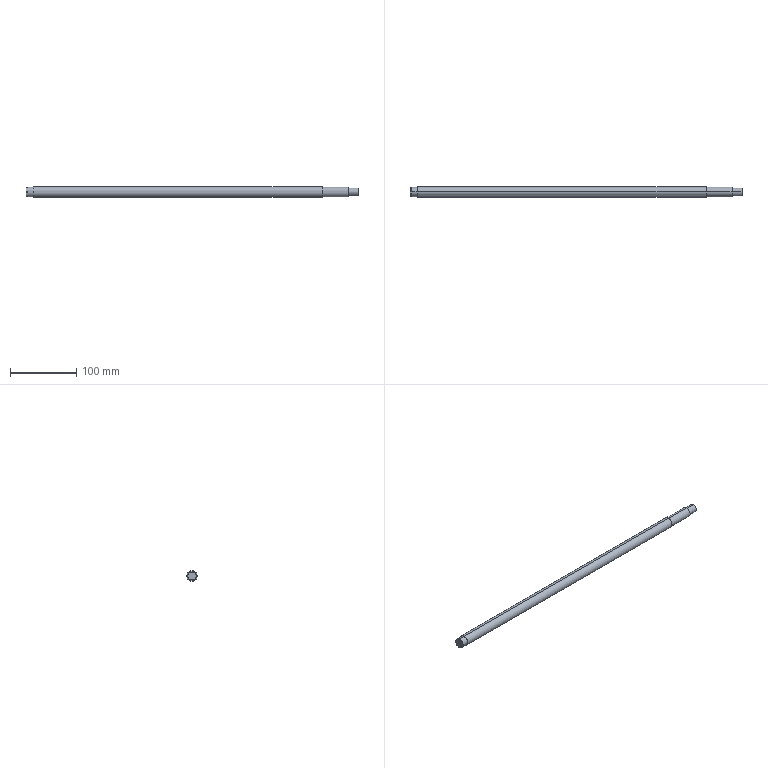Part | SolidWorks | features BaseBody 1 | 1 solid | 19 faces | box 500 x 16 x 16 mm | volume 97769 mm3 | cylinder 12 | plane 7 | commonest cylinder face diameters 14.3 x4 12 x2 12.3 x2 15 x2 16 x2
STEP:
#1=CARTESIAN_POINT('',(446.,0.,8.));
#2=VERTEX_POINT('',#1);
#3=CARTESIAN_POINT('',(446.,0.,-8.));
#4=VERTEX_POINT('',#3);
#5=CARTESIAN_POINT('',(446.,0.,0.));
#6=DIRECTION('',(-1.,0.,0.));
#7=DIRECTION('',(0.,0.,1.));
#8=AXIS2_PLACEMENT_3D('',#5,#6,#7);
#9=CIRCLE('',#8,8.);
#10=EDGE_CURVE('',#2,#4,#9,.T.);
#11=ORIENTED_EDGE('',*,*,#10,.T.);
#12=CARTESIAN_POINT('',(11.,0.,-8.));
#13=VERTEX_POINT('',#12);
#14=CARTESIAN_POINT('',(-271.923,0.,-8.));
#15=DIRECTION('',(-1.,0.,0.));
#16=VECTOR('',#15,1000.);
#17=LINE('',#14,#16);
#18=EDGE_CURVE('',#4,#13,#17,.T.);
#19=ORIENTED_EDGE('',*,*,#18,.T.);
#20=CARTESIAN_POINT('',(11.,0.,8.));
#21=VERTEX_POINT('',#20);
#22=CARTESIAN_POINT('',(11.,0.,0.));
#23=DIRECTION('',(1.,0.,0.));
#24=DIRECTION('',(0.,0.,1.));
#25=AXIS2_PLACEMENT_3D('',#22,#23,#24);
#26=CIRCLE('',#25,8.);
#27=EDGE_CURVE('',#13,#21,#26,.T.);
#28=ORIENTED_EDGE('',*,*,#27,.T.);
#29=CARTESIAN_POINT('',(-271.923,0.,8.));
#30=DIRECTION('',(-1.,0.,0.));
#31=VECTOR('',#30,1000.);
#32=LINE('',#29,#31);
#33=EDGE_CURVE('',#2,#21,#32,.T.);
#34=ORIENTED_EDGE('',*,*,#33,.F.);
#35=EDGE_LOOP('',(#11,#19,#28,#34));
#36=FACE_OUTER_BOUND('',#35,.T.);
#37=CARTESIAN_POINT('',(-271.923,0.,0.));
#38=DIRECTION('',(-1.,0.,0.));
#39=DIRECTION('',(0.,0.,1.));
#40=AXIS2_PLACEMENT_3D('',#37,#38,#39);
#41=CYLINDRICAL_SURFACE('',#40,8.);
#42=ADVANCED_FACE('',(#36),#41,.T.);
#43=CARTESIAN_POINT('',(11.,0.,7.15));
#44=VERTEX_POINT('',#43);
#45=CARTESIAN_POINT('',(11.,0.,-7.15));
#46=VERTEX_POINT('',#45);
#47=CARTESIAN_POINT('',(11.,0.,0.));
#48=DIRECTION('',(-1.,0.,0.));
#49=DIRECTION('',(0.,0.,1.));
#50=AXIS2_PLACEMENT_3D('',#47,#48,#49);
#51=CIRCLE('',#50,7.15);
#52=EDGE_CURVE('',#44,#46,#51,.T.);
#53=ORIENTED_EDGE('',*,*,#52,.T.);
#54=CARTESIAN_POINT('',(2.,0.,-7.15));
#55=VERTEX_POINT('',#54);
#56=CARTESIAN_POINT('',(-271.923,0.,-7.15));
#57=DIRECTION('',(-1.,0.,0.));
#58=VECTOR('',#57,1000.);
#59=LINE('',#56,#58);
#60=EDGE_CURVE('',#46,#55,#59,.T.);
#61=ORIENTED_EDGE('',*,*,#60,.T.);
#62=CARTESIAN_POINT('',(2.,0.,7.15));
#63=VERTEX_POINT('',#62);
#64=CARTESIAN_POINT('',(2.,0.,0.));
#65=DIRECTION('',(1.,0.,0.));
#66=DIRECTION('',(0.,0.,1.));
#67=AXIS2_PLACEMENT_3D('',#64,#65,#66);
#68=CIRCLE('',#67,7.15);
#69=EDGE_CURVE('',#55,#63,#68,.T.);
#70=ORIENTED_EDGE('',*,*,#69,.T.);
#71=CARTESIAN_POINT('',(-271.923,0.,7.15));
#72=DIRECTION('',(-1.,0.,0.));
#73=VECTOR('',#72,1000.);
#74=LINE('',#71,#73);
#75=EDGE_CURVE('',#44,#63,#74,.T.);
#76=ORIENTED_EDGE('',*,*,#75,.F.);
#77=EDGE_LOOP('',(#53,#61,#70,#76));
#78=FACE_OUTER_BOUND('',#77,.T.);
#79=CARTESIAN_POINT('',(-271.923,0.,0.));
#80=DIRECTION('',(-1.,0.,0.));
#81=DIRECTION('',(0.,0.,1.));
#82=AXIS2_PLACEMENT_3D('',#79,#80,#81);
#83=CYLINDRICAL_SURFACE('',#82,7.15);
#84=ADVANCED_FACE('',(#78),#83,.T.);
#85=CARTESIAN_POINT('',(485.,0.,7.5));
#86=VERTEX_POINT('',#85);
#87=CARTESIAN_POINT('',(485.,0.,-7.5));
#88=VERTEX_POINT('',#87);
#89=CARTESIAN_POINT('',(485.,0.,0.));
#90=DIRECTION('',(-1.,0.,0.));
#91=DIRECTION('',(0.,0.,1.));
#92=AXIS2_PLACEMENT_3D('',#89,#90,#91);
#93=CIRCLE('',#92,7.5);
#94=EDGE_CURVE('',#86,#88,#93,.T.);
#95=ORIENTED_EDGE('',*,*,#94,.T.);
#96=CARTESIAN_POINT('',(446.,0.,-7.5));
#97=VERTEX_POINT('',#96);
#98=CARTESIAN_POINT('',(-271.923,0.,-7.5));
#99=DIRECTION('',(-1.,0.,0.));
#100=VECTOR('',#99,1000.);
#101=LINE('',#98,#100);
#102=EDGE_CURVE('',#88,#97,#101,.T.);
#103=ORIENTED_EDGE('',*,*,#102,.T.);
#104=CARTESIAN_POINT('',(446.,0.,7.5));
#105=VERTEX_POINT('',#104);
#106=CARTESIAN_POINT('',(446.,0.,0.));
#107=DIRECTION('',(1.,0.,0.));
#108=DIRECTION('',(0.,0.,1.));
#109=AXIS2_PLACEMENT_3D('',#106,#107,#108);
#110=CIRCLE('',#109,7.5);
#111=EDGE_CURVE('',#97,#105,#110,.T.);
#112=ORIENTED_EDGE('',*,*,#111,.T.);
#113=CARTESIAN_POINT('',(-271.923,0.,7.5));
#114=DIRECTION('',(-1.,0.,0.));
#115=VECTOR('',#114,1000.);
#116=LINE('',#113,#115);
#117=EDGE_CURVE('',#86,#105,#116,.T.);
#118=ORIENTED_EDGE('',*,*,#117,.F.);
#119=EDGE_LOOP('',(#95,#103,#112,#118));
#120=FACE_OUTER_BOUND('',#119,.T.);
#121=CARTESIAN_POINT('',(-271.923,0.,0.));
#122=DIRECTION('',(-1.,0.,0.));
#123=DIRECTION('',(0.,0.,1.));
#124=AXIS2_PLACEMENT_3D('',#121,#122,#123);
#125=CYLINDRICAL_SURFACE('',#124,7.5);
#126=ADVANCED_FACE('',(#120),#125,.T.);
#127=CARTESIAN_POINT('',(2.,0.,6.15));
#128=VERTEX_POINT('',#127);
#129=CARTESIAN_POINT('',(2.,0.,-6.15));
#130=VERTEX_POINT('',#129);
#131=CARTESIAN_POINT('',(2.,0.,0.));
#132=DIRECTION('',(-1.,0.,0.));
#133=DIRECTION('',(0.,0.,1.));
#134=AXIS2_PLACEMENT_3D('',#131,#132,#133);
#135=CIRCLE('',#134,6.15);
#136=EDGE_CURVE('',#128,#130,#135,.T.);
#137=ORIENTED_EDGE('',*,*,#136,.T.);
#138=CARTESIAN_POINT('',(0.85,0.,-6.15));
#139=VERTEX_POINT('',#138);
#140=CARTESIAN_POINT('',(-271.923,0.,-6.15));
#141=DIRECTION('',(-1.,0.,0.));
#142=VECTOR('',#141,1000.);
#143=LINE('',#140,#142);
#144=EDGE_CURVE('',#130,#139,#143,.T.);
#145=ORIENTED_EDGE('',*,*,#144,.T.);
#146=CARTESIAN_POINT('',(0.85,0.,6.15));
#147=VERTEX_POINT('',#146);
#148=CARTESIAN_POINT('',(0.85,0.,0.));
#149=DIRECTION('',(1.,0.,0.));
#150=DIRECTION('',(0.,0.,1.));
#151=AXIS2_PLACEMENT_3D('',#148,#149,#150);
#152=CIRCLE('',#151,6.15);
#153=EDGE_CURVE('',#139,#147,#152,.T.);
#154=ORIENTED_EDGE('',*,*,#153,.T.);
#155=CARTESIAN_POINT('',(-271.923,0.,6.15));
#156=DIRECTION('',(-1.,0.,0.));
#157=VECTOR('',#156,1000.);
#158=LINE('',#155,#157);
#159=EDGE_CURVE('',#128,#147,#158,.T.);
#160=ORIENTED_EDGE('',*,*,#159,.F.);
#161=EDGE_LOOP('',(#137,#145,#154,#160));
#162=FACE_OUTER_BOUND('',#161,.T.);
#163=CARTESIAN_POINT('',(-271.923,0.,0.));
#164=DIRECTION('',(-1.,0.,0.));
#165=DIRECTION('',(0.,0.,1.));
#166=AXIS2_PLACEMENT_3D('',#163,#164,#165);
#167=CYLINDRICAL_SURFACE('',#166,6.15);
#168=ADVANCED_FACE('',(#162),#167,.T.);
#169=CARTESIAN_POINT('',(500.,0.,6.));
#170=VERTEX_POINT('',#169);
#171=CARTESIAN_POINT('',(500.,0.,-6.));
#172=VERTEX_POINT('',#171);
#173=CARTESIAN_POINT('',(500.,0.,0.));
#174=DIRECTION('',(-1.,0.,0.));
#175=DIRECTION('',(0.,0.,1.));
#176=AXIS2_PLACEMENT_3D('',#173,#174,#175);
#177=CIRCLE('',#176,6.);
#178=EDGE_CURVE('',#170,#172,#177,.T.);
#179=ORIENTED_EDGE('',*,*,#178,.T.);
#180=CARTESIAN_POINT('',(485.,0.,-6.));
#181=VERTEX_POINT('',#180);
#182=CARTESIAN_POINT('',(-271.923,0.,-6.));
#183=DIRECTION('',(-1.,0.,0.));
#184=VECTOR('',#183,1000.);
#185=LINE('',#182,#184);
#186=EDGE_CURVE('',#172,#181,#185,.T.);
#187=ORIENTED_EDGE('',*,*,#186,.T.);
#188=CARTESIAN_POINT('',(485.,0.,6.));
#189=VERTEX_POINT('',#188);
#190=CARTESIAN_POINT('',(485.,0.,0.));
#191=DIRECTION('',(1.,0.,0.));
#192=DIRECTION('',(0.,0.,1.));
#193=AXIS2_PLACEMENT_3D('',#190,#191,#192);
#194=CIRCLE('',#193,6.);
#195=EDGE_CURVE('',#181,#189,#194,.T.);
#196=ORIENTED_EDGE('',*,*,#195,.T.);
#197=CARTESIAN_POINT('',(-271.923,0.,6.));
#198=DIRECTION('',(-1.,0.,0.));
#199=VECTOR('',#198,1000.);
#200=LINE('',#197,#199);
#201=EDGE_CURVE('',#170,#189,#200,.T.);
#202=ORIENTED_EDGE('',*,*,#201,.F.);
#203=EDGE_LOOP('',(#179,#187,#196,#202));
#204=FACE_OUTER_BOUND('',#203,.T.);
#205=CARTESIAN_POINT('',(-271.923,0.,0.));
#206=DIRECTION('',(-1.,0.,0.));
#207=DIRECTION('',(0.,0.,1.));
#208=AXIS2_PLACEMENT_3D('',#205,#206,#207);
#209=CYLINDRICAL_SURFACE('',#208,6.);
#210=ADVANCED_FACE('',(#204),#209,.T.);
#211=CARTESIAN_POINT('',(0.85,0.,7.15));
#212=VERTEX_POINT('',#211);
#213=CARTESIAN_POINT('',(0.85,0.,-7.15));
#214=VERTEX_POINT('',#213);
#215=CARTESIAN_POINT('',(0.85,0.,0.));
#216=DIRECTION('',(-1.,0.,0.));
#217=DIRECTION('',(0.,0.,1.));
#218=AXIS2_PLACEMENT_3D('',#215,#216,#217);
#219=CIRCLE('',#218,7.15);
#220=EDGE_CURVE('',#212,#214,#219,.T.);
#221=ORIENTED_EDGE('',*,*,#220,.T.);
#222=CARTESIAN_POINT('',(0.,0.,-7.15));
#223=VERTEX_POINT('',#222);
#224=CARTESIAN_POINT('',(-271.923,0.,-7.15));
#225=DIRECTION('',(-1.,0.,0.));
#226=VECTOR('',#225,1000.);
#227=LINE('',#224,#226);
#228=EDGE_CURVE('',#214,#223,#227,.T.);
#229=ORIENTED_EDGE('',*,*,#228,.T.);
#230=CARTESIAN_POINT('',(0.,0.,7.15));
#231=VERTEX_POINT('',#230);
#232=CARTESIAN_POINT('',(0.,0.,0.));
#233=DIRECTION('',(1.,0.,0.));
#234=DIRECTION('',(0.,0.,1.));
#235=AXIS2_PLACEMENT_3D('',#232,#233,#234);
#236=CIRCLE('',#235,7.15);
#237=EDGE_CURVE('',#223,#231,#236,.T.);
#238=ORIENTED_EDGE('',*,*,#237,.T.);
#239=CARTESIAN_POINT('',(-271.923,0.,7.15));
#240=DIRECTION('',(-1.,0.,0.));
#241=VECTOR('',#240,1000.);
#242=LINE('',#239,#241);
#243=EDGE_CURVE('',#212,#231,#242,.T.);
#244=ORIENTED_EDGE('',*,*,#243,.F.);
#245=EDGE_LOOP('',(#221,#229,#238,#244));
#246=FACE_OUTER_BOUND('',#245,.T.);
#247=CARTESIAN_POINT('',(-271.923,0.,0.));
#248=DIRECTION('',(-1.,0.,0.));
#249=DIRECTION('',(0.,0.,1.));
#250=AXIS2_PLACEMENT_3D('',#247,#248,#249);
#251=CYLINDRICAL_SURFACE('',#250,7.15);
#252=ADVANCED_FACE('',(#246),#251,.T.);
#253=ORIENTED_EDGE('',*,*,#18,.F.);
#254=CARTESIAN_POINT('',(446.,0.,0.));
#255=DIRECTION('',(-1.,0.,0.));
#256=DIRECTION('',(0.,0.,1.));
#257=AXIS2_PLACEMENT_3D('',#254,#255,#256);
#258=CIRCLE('',#257,8.);
#259=EDGE_CURVE('',#4,#2,#258,.T.);
#260=ORIENTED_EDGE('',*,*,#259,.T.);
#261=ORIENTED_EDGE('',*,*,#33,.T.);
#262=CARTESIAN_POINT('',(11.,0.,0.));
#263=DIRECTION('',(1.,0.,0.));
#264=DIRECTION('',(0.,0.,1.));
#265=AXIS2_PLACEMENT_3D('',#262,#263,#264);
#266=CIRCLE('',#265,8.);
#267=EDGE_CURVE('',#21,#13,#266,.T.);
#268=ORIENTED_EDGE('',*,*,#267,.T.);
#269=EDGE_LOOP('',(#253,#260,#261,#268));
#270=FACE_OUTER_BOUND('',#269,.T.);
#271=CARTESIAN_POINT('',(-271.923,0.,0.));
#272=DIRECTION('',(-1.,0.,0.));
#273=DIRECTION('',(0.,0.,1.));
#274=AXIS2_PLACEMENT_3D('',#271,#272,#273);
#275=CYLINDRICAL_SURFACE('',#274,8.);
#276=ADVANCED_FACE('',(#270),#275,.T.);
#277=ORIENTED_EDGE('',*,*,#267,.F.);
#278=ORIENTED_EDGE('',*,*,#27,.F.);
#279=EDGE_LOOP('',(#277,#278));
#280=FACE_OUTER_BOUND('',#279,.T.);
#281=ORIENTED_EDGE('',*,*,#52,.F.);
#282=CARTESIAN_POINT('',(11.,0.,0.));
#283=DIRECTION('',(-1.,0.,0.));
#284=DIRECTION('',(0.,0.,1.));
#285=AXIS2_PLACEMENT_3D('',#282,#283,#284);
#286=CIRCLE('',#285,7.15);
#287=EDGE_CURVE('',#46,#44,#286,.T.);
#288=ORIENTED_EDGE('',*,*,#287,.F.);
#289=EDGE_LOOP('',(#281,#288));
#290=FACE_BOUND('',#289,.T.);
#291=CARTESIAN_POINT('',(11.,7.15,0.));
#292=DIRECTION('',(1.,0.,0.));
#293=DIRECTION('',(0.,0.,-1.));
#294=AXIS2_PLACEMENT_3D('',#291,#292,#293);
#295=PLANE('',#294);
#296=ADVANCED_FACE('',(#280,#290),#295,.F.);
#297=CARTESIAN_POINT('',(446.,0.,0.));
#298=DIRECTION('',(1.,0.,0.));
#299=DIRECTION('',(0.,0.,1.));
#300=AXIS2_PLACEMENT_3D('',#297,#298,#299);
#301=CIRCLE('',#300,7.5);
#302=EDGE_CURVE('',#105,#97,#301,.T.);
#303=ORIENTED_EDGE('',*,*,#302,.F.);
#304=ORIENTED_EDGE('',*,*,#111,.F.);
#305=EDGE_LOOP('',(#303,#304));
#306=FACE_BOUND('',#305,.T.);
#307=ORIENTED_EDGE('',*,*,#10,.F.);
#308=ORIENTED_EDGE('',*,*,#259,.F.);
#309=EDGE_LOOP('',(#307,#308));
#310=FACE_OUTER_BOUND('',#309,.T.);
#311=CARTESIAN_POINT('',(446.,8.,0.));
#312=DIRECTION('',(-1.,0.,0.));
#313=DIRECTION('',(0.,0.,1.));
#314=AXIS2_PLACEMENT_3D('',#311,#312,#313);
#315=PLANE('',#314);
#316=ADVANCED_FACE('',(#306,#310),#315,.F.);
#317=ORIENTED_EDGE('',*,*,#60,.F.);
#318=ORIENTED_EDGE('',*,*,#287,.T.);
#319=ORIENTED_EDGE('',*,*,#75,.T.);
#320=CARTESIAN_POINT('',(2.,0.,0.));
#321=DIRECTION('',(1.,0.,0.));
#322=DIRECTION('',(0.,0.,1.));
#323=AXIS2_PLACEMENT_3D('',#320,#321,#322);
#324=CIRCLE('',#323,7.15);
#325=EDGE_CURVE('',#63,#55,#324,.T.);
#326=ORIENTED_EDGE('',*,*,#325,.T.);
#327=EDGE_LOOP('',(#317,#318,#319,#326));
#328=FACE_OUTER_BOUND('',#327,.T.);
#329=CARTESIAN_POINT('',(-271.923,0.,0.));
#330=DIRECTION('',(-1.,0.,0.));
#331=DIRECTION('',(0.,0.,1.));
#332=AXIS2_PLACEMENT_3D('',#329,#330,#331);
#333=CYLINDRICAL_SURFACE('',#332,7.15);
#334=ADVANCED_FACE('',(#328),#333,.T.);
#335=ORIENTED_EDGE('',*,*,#102,.F.);
#336=CARTESIAN_POINT('',(485.,0.,0.));
#337=DIRECTION('',(-1.,0.,0.));
#338=DIRECTION('',(0.,0.,1.));
#339=AXIS2_PLACEMENT_3D('',#336,#337,#338);
#340=CIRCLE('',#339,7.5);
#341=EDGE_CURVE('',#88,#86,#340,.T.);
#342=ORIENTED_EDGE('',*,*,#341,.T.);
#343=ORIENTED_EDGE('',*,*,#117,.T.);
#344=ORIENTED_EDGE('',*,*,#302,.T.);
#345=EDGE_LOOP('',(#335,#342,#343,#344));
#346=FACE_OUTER_BOUND('',#345,.T.);
#347=CARTESIAN_POINT('',(-271.923,0.,0.));
#348=DIRECTION('',(-1.,0.,0.));
#349=DIRECTION('',(0.,0.,1.));
#350=AXIS2_PLACEMENT_3D('',#347,#348,#349);
#351=CYLINDRICAL_SURFACE('',#350,7.5);
#352=ADVANCED_FACE('',(#346),#351,.T.);
#353=ORIENTED_EDGE('',*,*,#325,.F.);
#354=ORIENTED_EDGE('',*,*,#69,.F.);
#355=EDGE_LOOP('',(#353,#354));
#356=FACE_OUTER_BOUND('',#355,.T.);
#357=ORIENTED_EDGE('',*,*,#136,.F.);
#358=CARTESIAN_POINT('',(2.,0.,0.));
#359=DIRECTION('',(-1.,0.,0.));
#360=DIRECTION('',(0.,0.,1.));
#361=AXIS2_PLACEMENT_3D('',#358,#359,#360);
#362=CIRCLE('',#361,6.15);
#363=EDGE_CURVE('',#130,#128,#362,.T.);
#364=ORIENTED_EDGE('',*,*,#363,.F.);
#365=EDGE_LOOP('',(#357,#364));
#366=FACE_BOUND('',#365,.T.);
#367=CARTESIAN_POINT('',(2.,6.15,0.));
#368=DIRECTION('',(1.,0.,0.));
#369=DIRECTION('',(0.,0.,-1.));
#370=AXIS2_PLACEMENT_3D('',#367,#368,#369);
#371=PLANE('',#370);
#372=ADVANCED_FACE('',(#356,#366),#371,.F.);
#373=CARTESIAN_POINT('',(485.,0.,0.));
#374=DIRECTION('',(1.,0.,0.));
#375=DIRECTION('',(0.,0.,1.));
#376=AXIS2_PLACEMENT_3D('',#373,#374,#375);
#377=CIRCLE('',#376,6.);
#378=EDGE_CURVE('',#189,#181,#377,.T.);
#379=ORIENTED_EDGE('',*,*,#378,.F.);
#380=ORIENTED_EDGE('',*,*,#195,.F.);
#381=EDGE_LOOP('',(#379,#380));
#382=FACE_BOUND('',#381,.T.);
#383=ORIENTED_EDGE('',*,*,#94,.F.);
#384=ORIENTED_EDGE('',*,*,#341,.F.);
#385=EDGE_LOOP('',(#383,#384));
#386=FACE_OUTER_BOUND('',#385,.T.);
#387=CARTESIAN_POINT('',(485.,7.5,0.));
#388=DIRECTION('',(-1.,0.,0.));
#389=DIRECTION('',(0.,0.,1.));
#390=AXIS2_PLACEMENT_3D('',#387,#388,#389);
#391=PLANE('',#390);
#392=ADVANCED_FACE('',(#382,#386),#391,.F.);
#393=ORIENTED_EDGE('',*,*,#144,.F.);
#394=ORIENTED_EDGE('',*,*,#363,.T.);
#395=ORIENTED_EDGE('',*,*,#159,.T.);
#396=CARTESIAN_POINT('',(0.85,0.,0.));
#397=DIRECTION('',(1.,0.,0.));
#398=DIRECTION('',(0.,0.,1.));
#399=AXIS2_PLACEMENT_3D('',#396,#397,#398);
#400=CIRCLE('',#399,6.15);
#401=EDGE_CURVE('',#147,#139,#400,.T.);
#402=ORIENTED_EDGE('',*,*,#401,.T.);
#403=EDGE_LOOP('',(#393,#394,#395,#402));
#404=FACE_OUTER_BOUND('',#403,.T.);
#405=CARTESIAN_POINT('',(-271.923,0.,0.));
#406=DIRECTION('',(-1.,0.,0.));
#407=DIRECTION('',(0.,0.,1.));
#408=AXIS2_PLACEMENT_3D('',#405,#406,#407);
#409=CYLINDRICAL_SURFACE('',#408,6.15);
#410=ADVANCED_FACE('',(#404),#409,.T.);
#411=ORIENTED_EDGE('',*,*,#186,.F.);
#412=CARTESIAN_POINT('',(500.,0.,0.));
#413=DIRECTION('',(-1.,0.,0.));
#414=DIRECTION('',(0.,0.,1.));
#415=AXIS2_PLACEMENT_3D('',#412,#413,#414);
#416=CIRCLE('',#415,6.);
#417=EDGE_CURVE('',#172,#170,#416,.T.);
#418=ORIENTED_EDGE('',*,*,#417,.T.);
#419=ORIENTED_EDGE('',*,*,#201,.T.);
#420=ORIENTED_EDGE('',*,*,#378,.T.);
#421=EDGE_LOOP('',(#411,#418,#419,#420));
#422=FACE_OUTER_BOUND('',#421,.T.);
#423=CARTESIAN_POINT('',(-271.923,0.,0.));
#424=DIRECTION('',(-1.,0.,0.));
#425=DIRECTION('',(0.,0.,1.));
#426=AXIS2_PLACEMENT_3D('',#423,#424,#425);
#427=CYLINDRICAL_SURFACE('',#426,6.);
#428=ADVANCED_FACE('',(#422),#427,.T.);
#429=ORIENTED_EDGE('',*,*,#401,.F.);
#430=ORIENTED_EDGE('',*,*,#153,.F.);
#431=EDGE_LOOP('',(#429,#430));
#432=FACE_BOUND('',#431,.T.);
#433=ORIENTED_EDGE('',*,*,#220,.F.);
#434=CARTESIAN_POINT('',(0.85,0.,0.));
#435=DIRECTION('',(-1.,0.,0.));
#436=DIRECTION('',(0.,0.,1.));
#437=AXIS2_PLACEMENT_3D('',#434,#435,#436);
#438=CIRCLE('',#437,7.15);
#439=EDGE_CURVE('',#214,#212,#438,.T.);
#440=ORIENTED_EDGE('',*,*,#439,.F.);
#441=EDGE_LOOP('',(#433,#440));
#442=FACE_OUTER_BOUND('',#441,.T.);
#443=CARTESIAN_POINT('',(0.85,7.15,0.));
#444=DIRECTION('',(-1.,0.,0.));
#445=DIRECTION('',(0.,0.,1.));
#446=AXIS2_PLACEMENT_3D('',#443,#444,#445);
#447=PLANE('',#446);
#448=ADVANCED_FACE('',(#432,#442),#447,.F.);
#449=ORIENTED_EDGE('',*,*,#178,.F.);
#450=ORIENTED_EDGE('',*,*,#417,.F.);
#451=EDGE_LOOP('',(#449,#450));
#452=FACE_OUTER_BOUND('',#451,.T.);
#453=CARTESIAN_POINT('',(500.,6.,0.));
#454=DIRECTION('',(-1.,0.,0.));
#455=DIRECTION('',(0.,0.,1.));
#456=AXIS2_PLACEMENT_3D('',#453,#454,#455);
#457=PLANE('',#456);
#458=ADVANCED_FACE('',(#452),#457,.F.);
#459=ORIENTED_EDGE('',*,*,#228,.F.);
#460=ORIENTED_EDGE('',*,*,#439,.T.);
#461=ORIENTED_EDGE('',*,*,#243,.T.);
#462=CARTESIAN_POINT('',(0.,0.,0.));
#463=DIRECTION('',(1.,0.,0.));
#464=DIRECTION('',(0.,0.,1.));
#465=AXIS2_PLACEMENT_3D('',#462,#463,#464);
#466=CIRCLE('',#465,7.15);
#467=EDGE_CURVE('',#231,#223,#466,.T.);
#468=ORIENTED_EDGE('',*,*,#467,.T.);
#469=EDGE_LOOP('',(#459,#460,#461,#468));
#470=FACE_OUTER_BOUND('',#469,.T.);
#471=CARTESIAN_POINT('',(-271.923,0.,0.));
#472=DIRECTION('',(-1.,0.,0.));
#473=DIRECTION('',(0.,0.,1.));
#474=AXIS2_PLACEMENT_3D('',#471,#472,#473);
#475=CYLINDRICAL_SURFACE('',#474,7.15);
#476=ADVANCED_FACE('',(#470),#475,.T.);
#477=ORIENTED_EDGE('',*,*,#467,.F.);
#478=ORIENTED_EDGE('',*,*,#237,.F.);
#479=EDGE_LOOP('',(#477,#478));
#480=FACE_OUTER_BOUND('',#479,.T.);
#481=CARTESIAN_POINT('',(0.,0.,0.));
#482=DIRECTION('',(1.,0.,0.));
#483=DIRECTION('',(0.,0.,-1.));
#484=AXIS2_PLACEMENT_3D('',#481,#482,#483);
#485=PLANE('',#484);
#486=ADVANCED_FACE('',(#480),#485,.F.);
#487=CLOSED_SHELL('',(#42,#84,#126,#168,#210,#252,#276,#296,#316,#334,#352,#372,#392,#410,#428,#448,#458,#476,#486));
#488=MANIFOLD_SOLID_BREP('',#487);
#489=CARTESIAN_POINT('',(0.,0.,0.));
#490=DIRECTION('',(0.,0.,1.));
#491=DIRECTION('',(1.,0.,0.));
#492=AXIS2_PLACEMENT_3D('',#489,#490,#491);
#493=(LENGTH_UNIT()NAMED_UNIT(*)SI_UNIT(.MILLI.,.METRE.));
#494=UNCERTAINTY_MEASURE_WITH_UNIT(LENGTH_MEASURE(0.00001),#493,'','');
#495=(NAMED_UNIT(*)PLANE_ANGLE_UNIT()SI_UNIT($,.RADIAN.));
#496=(NAMED_UNIT(*)SI_UNIT($,.STERADIAN.)SOLID_ANGLE_UNIT());
#497=(GEOMETRIC_REPRESENTATION_CONTEXT(3)GLOBAL_UNCERTAINTY_ASSIGNED_CONTEXT((#494))GLOBAL_UNIT_ASSIGNED_CONTEXT((#493,#495,#496))REPRESENTATION_CONTEXT('',''));
#498=ADVANCED_BREP_SHAPE_REPRESENTATION('',(#488,#492),#497);